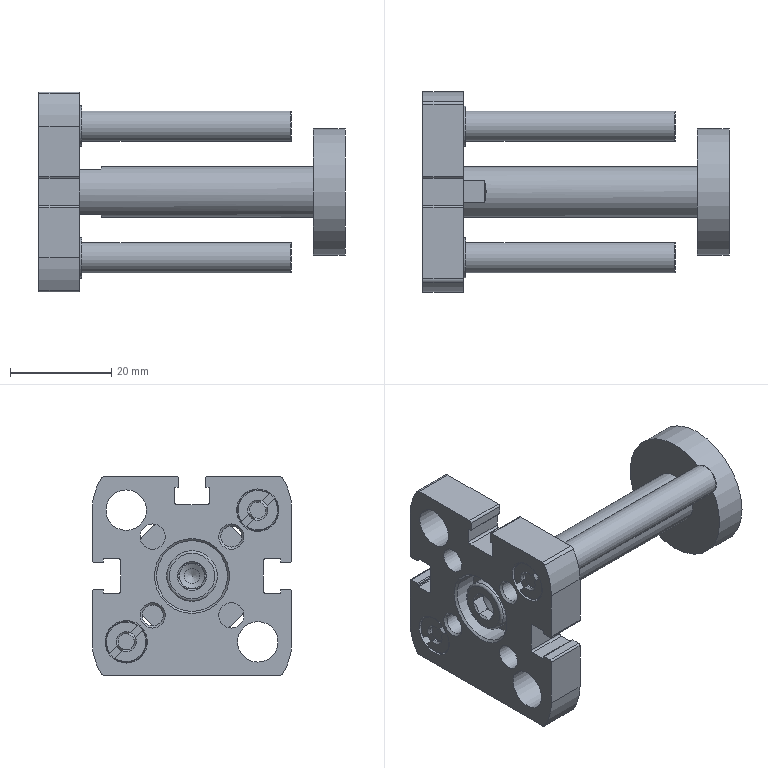Part | NX | features BREP 1 | 1 solid | 171 faces | box 60.5 x 39.5 x 39.5 mm | volume 18607 mm3 | plane 80 | cylinder 63 | cone 25 | torus 3 | commonest cylinder face diameters 0.4 x12 0.8 x12 8 x6 1.6 x4 3.242 x4 4 x4